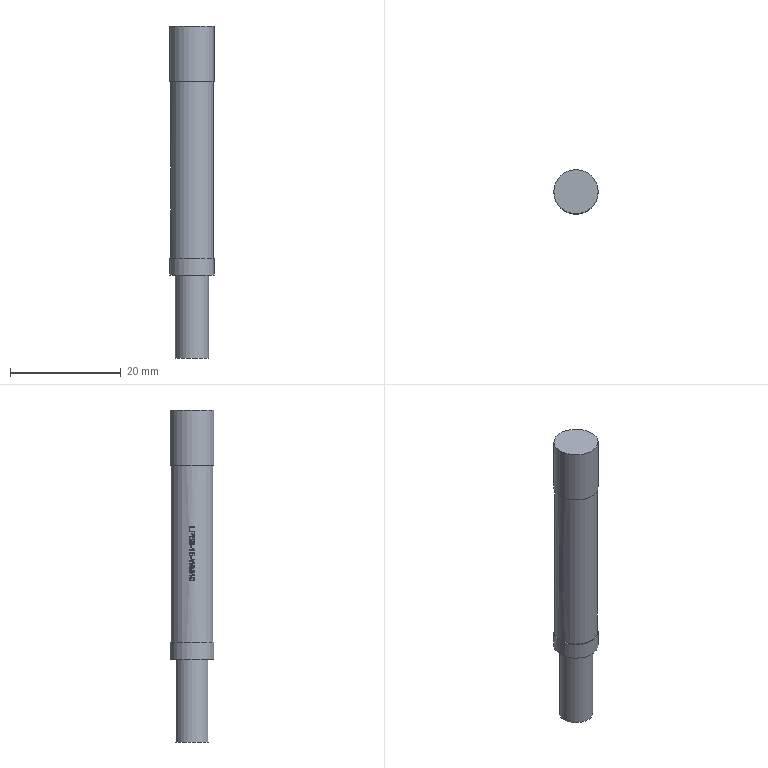Part | STEP file | LPS 2-10_id898_x_t | 1 solid | 174 faces | box 8 x 8 x 60 mm | volume 2567 mm3 | plane 88 | other 71 | cylinder 15 | commonest cylinder face diameters 7.7 x12 8 x2 6 x1